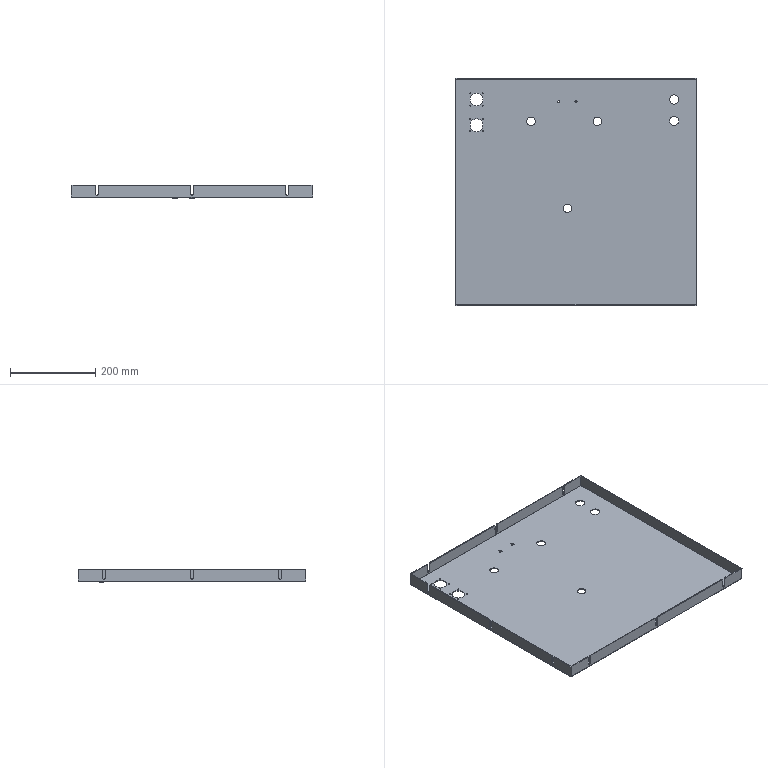Part | STEP file | 1 solid | 136 faces | box 566 x 533 x 32 mm | volume 714825 mm3 | cylinder 73 | plane 63 | commonest cylinder face diameters 4 x18 2.5 x16 7 x9 20 x6 0.2 x4 4.2 x4